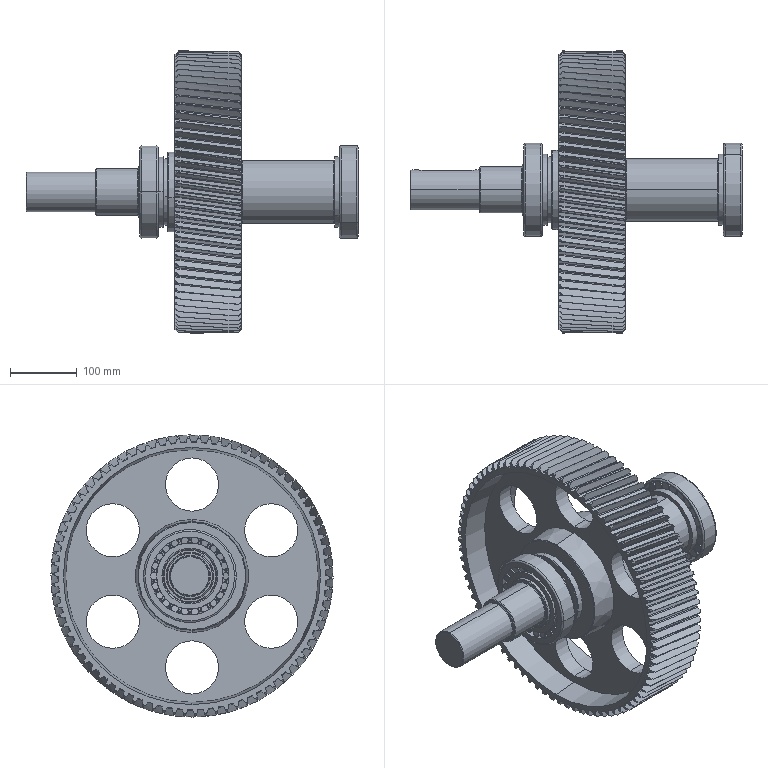Part | SolidWorks | 6 solids | 1194 faces | box 499.25 x 424.15 x 424.15 mm | volume 7884570 mm3 | spline 410 | cone 310 | torus 202 | cylinder 143 | plane 129 | commonest cylinder face diameters 424.15 x83 80 x22 22 x5 85 x5 99.889 x4 106.711 x4